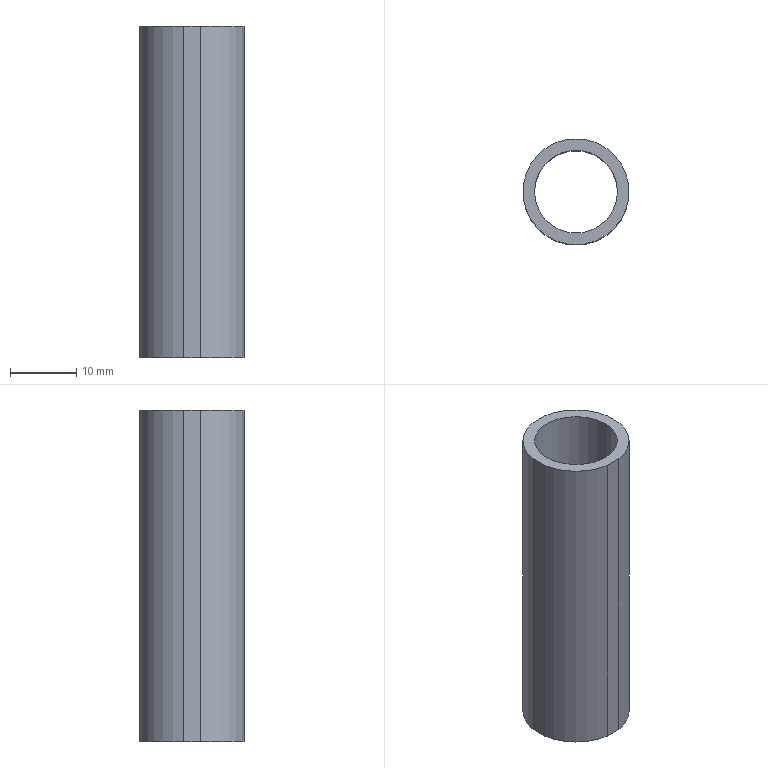Part | SolidWorks | features Extrusion 1, ICE 1 | 1 solid | 12 faces | box 15.8 x 15.8 x 50 mm | volume 3884 mm3 | cylinder 6 | plane 6 | commonest cylinder face diameters 16 x4 12.5 x2
STEP:
#1=CARTESIAN_POINT('',(-6.25,0.,50.));
#2=VERTEX_POINT('',#1);
#3=CARTESIAN_POINT('',(6.25,0.,50.));
#4=VERTEX_POINT('',#3);
#5=CARTESIAN_POINT('',(0.,0.,50.));
#6=DIRECTION('',(0.,0.,1.));
#7=DIRECTION('',(1.,0.,0.));
#8=AXIS2_PLACEMENT_3D('',#5,#6,#7);
#9=CIRCLE('',#8,6.25);
#10=EDGE_CURVE('',#2,#4,#9,.T.);
#11=ORIENTED_EDGE('',*,*,#10,.T.);
#12=CARTESIAN_POINT('',(6.25,0.,0.));
#13=VERTEX_POINT('',#12);
#14=CARTESIAN_POINT('',(6.25,0.,50.));
#15=DIRECTION('',(0.,0.,-1.));
#16=VECTOR('',#15,1000.);
#17=LINE('',#14,#16);
#18=EDGE_CURVE('',#4,#13,#17,.T.);
#19=ORIENTED_EDGE('',*,*,#18,.T.);
#20=CARTESIAN_POINT('',(-6.25,0.,0.));
#21=VERTEX_POINT('',#20);
#22=CARTESIAN_POINT('',(0.,0.,0.));
#23=DIRECTION('',(0.,0.,1.));
#24=DIRECTION('',(1.,0.,0.));
#25=AXIS2_PLACEMENT_3D('',#22,#23,#24);
#26=CIRCLE('',#25,6.25);
#27=EDGE_CURVE('',#21,#13,#26,.T.);
#28=ORIENTED_EDGE('',*,*,#27,.F.);
#29=CARTESIAN_POINT('',(-6.25,0.,50.));
#30=DIRECTION('',(0.,0.,-1.));
#31=VECTOR('',#30,1000.);
#32=LINE('',#29,#31);
#33=EDGE_CURVE('',#2,#21,#32,.T.);
#34=ORIENTED_EDGE('',*,*,#33,.F.);
#35=EDGE_LOOP('',(#11,#19,#28,#34));
#36=FACE_OUTER_BOUND('',#35,.T.);
#37=CARTESIAN_POINT('',(0.,0.,50.));
#38=DIRECTION('',(0.,0.,-1.));
#39=DIRECTION('',(-1.,0.,0.));
#40=AXIS2_PLACEMENT_3D('',#37,#38,#39);
#41=CYLINDRICAL_SURFACE('',#40,6.25);
#42=ADVANCED_FACE('',(#36),#41,.F.);
#43=ORIENTED_EDGE('',*,*,#10,.F.);
#44=CARTESIAN_POINT('',(0.,0.,50.));
#45=DIRECTION('',(0.,0.,1.));
#46=DIRECTION('',(1.,0.,0.));
#47=AXIS2_PLACEMENT_3D('',#44,#45,#46);
#48=CIRCLE('',#47,6.25);
#49=EDGE_CURVE('',#4,#2,#48,.T.);
#50=ORIENTED_EDGE('',*,*,#49,.F.);
#51=EDGE_LOOP('',(#43,#50));
#52=FACE_BOUND('',#51,.T.);
#53=CARTESIAN_POINT('',(-1.261,7.9,50.));
#54=VERTEX_POINT('',#53);
#55=CARTESIAN_POINT('',(-7.9,1.261,50.));
#56=VERTEX_POINT('',#55);
#57=CARTESIAN_POINT('',(0.,0.,50.));
#58=DIRECTION('',(0.,0.,1.));
#59=DIRECTION('',(1.,0.,0.));
#60=AXIS2_PLACEMENT_3D('',#57,#58,#59);
#61=CIRCLE('',#60,8.);
#62=EDGE_CURVE('',#54,#56,#61,.T.);
#63=ORIENTED_EDGE('',*,*,#62,.T.);
#64=CARTESIAN_POINT('',(-7.9,-1.261,50.));
#65=VERTEX_POINT('',#64);
#66=CARTESIAN_POINT('',(-7.9,7.9,50.));
#67=DIRECTION('',(0.,-1.,0.));
#68=VECTOR('',#67,1000.);
#69=LINE('',#66,#68);
#70=EDGE_CURVE('',#56,#65,#69,.T.);
#71=ORIENTED_EDGE('',*,*,#70,.T.);
#72=CARTESIAN_POINT('',(-1.261,-7.9,50.));
#73=VERTEX_POINT('',#72);
#74=CARTESIAN_POINT('',(0.,0.,50.));
#75=DIRECTION('',(0.,0.,1.));
#76=DIRECTION('',(1.,0.,0.));
#77=AXIS2_PLACEMENT_3D('',#74,#75,#76);
#78=CIRCLE('',#77,8.);
#79=EDGE_CURVE('',#65,#73,#78,.T.);
#80=ORIENTED_EDGE('',*,*,#79,.T.);
#81=CARTESIAN_POINT('',(1.261,-7.9,50.));
#82=VERTEX_POINT('',#81);
#83=CARTESIAN_POINT('',(7.9,-7.9,50.));
#84=DIRECTION('',(1.,0.,0.));
#85=VECTOR('',#84,1000.);
#86=LINE('',#83,#85);
#87=EDGE_CURVE('',#73,#82,#86,.T.);
#88=ORIENTED_EDGE('',*,*,#87,.T.);
#89=CARTESIAN_POINT('',(7.9,-1.261,50.));
#90=VERTEX_POINT('',#89);
#91=CARTESIAN_POINT('',(0.,0.,50.));
#92=DIRECTION('',(0.,0.,1.));
#93=DIRECTION('',(1.,0.,0.));
#94=AXIS2_PLACEMENT_3D('',#91,#92,#93);
#95=CIRCLE('',#94,8.);
#96=EDGE_CURVE('',#82,#90,#95,.T.);
#97=ORIENTED_EDGE('',*,*,#96,.T.);
#98=CARTESIAN_POINT('',(7.9,1.261,50.));
#99=VERTEX_POINT('',#98);
#100=CARTESIAN_POINT('',(7.9,7.9,50.));
#101=DIRECTION('',(0.,1.,0.));
#102=VECTOR('',#101,1000.);
#103=LINE('',#100,#102);
#104=EDGE_CURVE('',#90,#99,#103,.T.);
#105=ORIENTED_EDGE('',*,*,#104,.T.);
#106=CARTESIAN_POINT('',(1.261,7.9,50.));
#107=VERTEX_POINT('',#106);
#108=CARTESIAN_POINT('',(0.,0.,50.));
#109=DIRECTION('',(0.,0.,1.));
#110=DIRECTION('',(1.,0.,0.));
#111=AXIS2_PLACEMENT_3D('',#108,#109,#110);
#112=CIRCLE('',#111,8.);
#113=EDGE_CURVE('',#99,#107,#112,.T.);
#114=ORIENTED_EDGE('',*,*,#113,.T.);
#115=CARTESIAN_POINT('',(7.9,7.9,50.));
#116=DIRECTION('',(-1.,0.,0.));
#117=VECTOR('',#116,1000.);
#118=LINE('',#115,#117);
#119=EDGE_CURVE('',#107,#54,#118,.T.);
#120=ORIENTED_EDGE('',*,*,#119,.T.);
#121=EDGE_LOOP('',(#63,#71,#80,#88,#97,#105,#114,#120));
#122=FACE_OUTER_BOUND('',#121,.T.);
#123=CARTESIAN_POINT('',(0.,0.,50.));
#124=DIRECTION('',(0.,0.,1.));
#125=DIRECTION('',(1.,0.,0.));
#126=AXIS2_PLACEMENT_3D('',#123,#124,#125);
#127=PLANE('',#126);
#128=ADVANCED_FACE('',(#52,#122),#127,.T.);
#129=ORIENTED_EDGE('',*,*,#27,.T.);
#130=CARTESIAN_POINT('',(0.,0.,0.));
#131=DIRECTION('',(0.,0.,1.));
#132=DIRECTION('',(1.,0.,0.));
#133=AXIS2_PLACEMENT_3D('',#130,#131,#132);
#134=CIRCLE('',#133,6.25);
#135=EDGE_CURVE('',#13,#21,#134,.T.);
#136=ORIENTED_EDGE('',*,*,#135,.T.);
#137=EDGE_LOOP('',(#129,#136));
#138=FACE_BOUND('',#137,.T.);
#139=CARTESIAN_POINT('',(-7.9,1.261,0.));
#140=VERTEX_POINT('',#139);
#141=CARTESIAN_POINT('',(-7.9,-1.261,0.));
#142=VERTEX_POINT('',#141);
#143=CARTESIAN_POINT('',(-7.9,7.9,0.));
#144=DIRECTION('',(0.,-1.,0.));
#145=VECTOR('',#144,1000.);
#146=LINE('',#143,#145);
#147=EDGE_CURVE('',#140,#142,#146,.T.);
#148=ORIENTED_EDGE('',*,*,#147,.F.);
#149=CARTESIAN_POINT('',(-1.261,7.9,0.));
#150=VERTEX_POINT('',#149);
#151=CARTESIAN_POINT('',(0.,0.,0.));
#152=DIRECTION('',(0.,0.,1.));
#153=DIRECTION('',(1.,0.,0.));
#154=AXIS2_PLACEMENT_3D('',#151,#152,#153);
#155=CIRCLE('',#154,8.);
#156=EDGE_CURVE('',#150,#140,#155,.T.);
#157=ORIENTED_EDGE('',*,*,#156,.F.);
#158=CARTESIAN_POINT('',(1.261,7.9,0.));
#159=VERTEX_POINT('',#158);
#160=CARTESIAN_POINT('',(7.9,7.9,0.));
#161=DIRECTION('',(-1.,0.,0.));
#162=VECTOR('',#161,1000.);
#163=LINE('',#160,#162);
#164=EDGE_CURVE('',#159,#150,#163,.T.);
#165=ORIENTED_EDGE('',*,*,#164,.F.);
#166=CARTESIAN_POINT('',(7.9,1.261,0.));
#167=VERTEX_POINT('',#166);
#168=CARTESIAN_POINT('',(0.,0.,0.));
#169=DIRECTION('',(0.,0.,1.));
#170=DIRECTION('',(1.,0.,0.));
#171=AXIS2_PLACEMENT_3D('',#168,#169,#170);
#172=CIRCLE('',#171,8.);
#173=EDGE_CURVE('',#167,#159,#172,.T.);
#174=ORIENTED_EDGE('',*,*,#173,.F.);
#175=CARTESIAN_POINT('',(7.9,-1.261,0.));
#176=VERTEX_POINT('',#175);
#177=CARTESIAN_POINT('',(7.9,7.9,0.));
#178=DIRECTION('',(0.,1.,0.));
#179=VECTOR('',#178,1000.);
#180=LINE('',#177,#179);
#181=EDGE_CURVE('',#176,#167,#180,.T.);
#182=ORIENTED_EDGE('',*,*,#181,.F.);
#183=CARTESIAN_POINT('',(1.261,-7.9,0.));
#184=VERTEX_POINT('',#183);
#185=CARTESIAN_POINT('',(0.,0.,0.));
#186=DIRECTION('',(0.,0.,1.));
#187=DIRECTION('',(1.,0.,0.));
#188=AXIS2_PLACEMENT_3D('',#185,#186,#187);
#189=CIRCLE('',#188,8.);
#190=EDGE_CURVE('',#184,#176,#189,.T.);
#191=ORIENTED_EDGE('',*,*,#190,.F.);
#192=CARTESIAN_POINT('',(-1.261,-7.9,0.));
#193=VERTEX_POINT('',#192);
#194=CARTESIAN_POINT('',(7.9,-7.9,0.));
#195=DIRECTION('',(1.,0.,0.));
#196=VECTOR('',#195,1000.);
#197=LINE('',#194,#196);
#198=EDGE_CURVE('',#193,#184,#197,.T.);
#199=ORIENTED_EDGE('',*,*,#198,.F.);
#200=CARTESIAN_POINT('',(0.,0.,0.));
#201=DIRECTION('',(0.,0.,1.));
#202=DIRECTION('',(1.,0.,0.));
#203=AXIS2_PLACEMENT_3D('',#200,#201,#202);
#204=CIRCLE('',#203,8.);
#205=EDGE_CURVE('',#142,#193,#204,.T.);
#206=ORIENTED_EDGE('',*,*,#205,.F.);
#207=EDGE_LOOP('',(#148,#157,#165,#174,#182,#191,#199,#206));
#208=FACE_OUTER_BOUND('',#207,.T.);
#209=CARTESIAN_POINT('',(0.,0.,0.));
#210=DIRECTION('',(0.,0.,1.));
#211=DIRECTION('',(1.,0.,0.));
#212=AXIS2_PLACEMENT_3D('',#209,#210,#211);
#213=PLANE('',#212);
#214=ADVANCED_FACE('',(#138,#208),#213,.F.);
#215=CARTESIAN_POINT('',(-7.9,1.261,50.));
#216=DIRECTION('',(0.,0.,-1.));
#217=VECTOR('',#216,1000.);
#218=LINE('',#215,#217);
#219=EDGE_CURVE('',#56,#140,#218,.T.);
#220=ORIENTED_EDGE('',*,*,#219,.F.);
#221=ORIENTED_EDGE('',*,*,#62,.F.);
#222=CARTESIAN_POINT('',(-1.261,7.9,50.));
#223=DIRECTION('',(0.,0.,1.));
#224=VECTOR('',#223,1000.);
#225=LINE('',#222,#224);
#226=EDGE_CURVE('',#150,#54,#225,.T.);
#227=ORIENTED_EDGE('',*,*,#226,.F.);
#228=ORIENTED_EDGE('',*,*,#156,.T.);
#229=EDGE_LOOP('',(#220,#221,#227,#228));
#230=FACE_OUTER_BOUND('',#229,.T.);
#231=CARTESIAN_POINT('',(0.,0.,50.));
#232=DIRECTION('',(0.,0.,-1.));
#233=DIRECTION('',(-1.,0.,0.));
#234=AXIS2_PLACEMENT_3D('',#231,#232,#233);
#235=CYLINDRICAL_SURFACE('',#234,8.);
#236=ADVANCED_FACE('',(#230),#235,.T.);
#237=CARTESIAN_POINT('',(-7.9,-1.261,50.));
#238=DIRECTION('',(0.,0.,1.));
#239=VECTOR('',#238,1000.);
#240=LINE('',#237,#239);
#241=EDGE_CURVE('',#142,#65,#240,.T.);
#242=ORIENTED_EDGE('',*,*,#241,.F.);
#243=ORIENTED_EDGE('',*,*,#205,.T.);
#244=CARTESIAN_POINT('',(-1.261,-7.9,50.));
#245=DIRECTION('',(0.,0.,-1.));
#246=VECTOR('',#245,1000.);
#247=LINE('',#244,#246);
#248=EDGE_CURVE('',#73,#193,#247,.T.);
#249=ORIENTED_EDGE('',*,*,#248,.F.);
#250=ORIENTED_EDGE('',*,*,#79,.F.);
#251=EDGE_LOOP('',(#242,#243,#249,#250));
#252=FACE_OUTER_BOUND('',#251,.T.);
#253=CARTESIAN_POINT('',(0.,0.,50.));
#254=DIRECTION('',(0.,0.,-1.));
#255=DIRECTION('',(-1.,0.,0.));
#256=AXIS2_PLACEMENT_3D('',#253,#254,#255);
#257=CYLINDRICAL_SURFACE('',#256,8.);
#258=ADVANCED_FACE('',(#252),#257,.T.);
#259=CARTESIAN_POINT('',(1.261,7.9,50.));
#260=DIRECTION('',(0.,0.,-1.));
#261=VECTOR('',#260,1000.);
#262=LINE('',#259,#261);
#263=EDGE_CURVE('',#107,#159,#262,.T.);
#264=ORIENTED_EDGE('',*,*,#263,.F.);
#265=ORIENTED_EDGE('',*,*,#113,.F.);
#266=CARTESIAN_POINT('',(7.9,1.261,50.));
#267=DIRECTION('',(0.,0.,1.));
#268=VECTOR('',#267,1000.);
#269=LINE('',#266,#268);
#270=EDGE_CURVE('',#167,#99,#269,.T.);
#271=ORIENTED_EDGE('',*,*,#270,.F.);
#272=ORIENTED_EDGE('',*,*,#173,.T.);
#273=EDGE_LOOP('',(#264,#265,#271,#272));
#274=FACE_OUTER_BOUND('',#273,.T.);
#275=CARTESIAN_POINT('',(0.,0.,50.));
#276=DIRECTION('',(0.,0.,-1.));
#277=DIRECTION('',(-1.,0.,0.));
#278=AXIS2_PLACEMENT_3D('',#275,#276,#277);
#279=CYLINDRICAL_SURFACE('',#278,8.);
#280=ADVANCED_FACE('',(#274),#279,.T.);
#281=CARTESIAN_POINT('',(7.9,-1.261,50.));
#282=DIRECTION('',(0.,0.,-1.));
#283=VECTOR('',#282,1000.);
#284=LINE('',#281,#283);
#285=EDGE_CURVE('',#90,#176,#284,.T.);
#286=ORIENTED_EDGE('',*,*,#285,.F.);
#287=ORIENTED_EDGE('',*,*,#96,.F.);
#288=CARTESIAN_POINT('',(1.261,-7.9,50.));
#289=DIRECTION('',(0.,0.,1.));
#290=VECTOR('',#289,1000.);
#291=LINE('',#288,#290);
#292=EDGE_CURVE('',#184,#82,#291,.T.);
#293=ORIENTED_EDGE('',*,*,#292,.F.);
#294=ORIENTED_EDGE('',*,*,#190,.T.);
#295=EDGE_LOOP('',(#286,#287,#293,#294));
#296=FACE_OUTER_BOUND('',#295,.T.);
#297=CARTESIAN_POINT('',(0.,0.,50.));
#298=DIRECTION('',(0.,0.,-1.));
#299=DIRECTION('',(-1.,0.,0.));
#300=AXIS2_PLACEMENT_3D('',#297,#298,#299);
#301=CYLINDRICAL_SURFACE('',#300,8.);
#302=ADVANCED_FACE('',(#296),#301,.T.);
#303=ORIENTED_EDGE('',*,*,#18,.F.);
#304=ORIENTED_EDGE('',*,*,#49,.T.);
#305=ORIENTED_EDGE('',*,*,#33,.T.);
#306=ORIENTED_EDGE('',*,*,#135,.F.);
#307=EDGE_LOOP('',(#303,#304,#305,#306));
#308=FACE_OUTER_BOUND('',#307,.T.);
#309=CARTESIAN_POINT('',(0.,0.,50.));
#310=DIRECTION('',(0.,0.,-1.));
#311=DIRECTION('',(-1.,0.,0.));
#312=AXIS2_PLACEMENT_3D('',#309,#310,#311);
#313=CYLINDRICAL_SURFACE('',#312,6.25);
#314=ADVANCED_FACE('',(#308),#313,.F.);
#315=ORIENTED_EDGE('',*,*,#248,.T.);
#316=ORIENTED_EDGE('',*,*,#198,.T.);
#317=ORIENTED_EDGE('',*,*,#292,.T.);
#318=ORIENTED_EDGE('',*,*,#87,.F.);
#319=EDGE_LOOP('',(#315,#316,#317,#318));
#320=FACE_OUTER_BOUND('',#319,.T.);
#321=CARTESIAN_POINT('',(7.9,-7.9,0.));
#322=DIRECTION('',(0.,-1.,0.));
#323=DIRECTION('',(1.,0.,0.));
#324=AXIS2_PLACEMENT_3D('',#321,#322,#323);
#325=PLANE('',#324);
#326=ADVANCED_FACE('',(#320),#325,.T.);
#327=ORIENTED_EDGE('',*,*,#285,.T.);
#328=ORIENTED_EDGE('',*,*,#181,.T.);
#329=ORIENTED_EDGE('',*,*,#270,.T.);
#330=ORIENTED_EDGE('',*,*,#104,.F.);
#331=EDGE_LOOP('',(#327,#328,#329,#330));
#332=FACE_OUTER_BOUND('',#331,.T.);
#333=CARTESIAN_POINT('',(7.9,7.9,0.));
#334=DIRECTION('',(1.,0.,0.));
#335=DIRECTION('',(0.,1.,0.));
#336=AXIS2_PLACEMENT_3D('',#333,#334,#335);
#337=PLANE('',#336);
#338=ADVANCED_FACE('',(#332),#337,.T.);
#339=ORIENTED_EDGE('',*,*,#263,.T.);
#340=ORIENTED_EDGE('',*,*,#164,.T.);
#341=ORIENTED_EDGE('',*,*,#226,.T.);
#342=ORIENTED_EDGE('',*,*,#119,.F.);
#343=EDGE_LOOP('',(#339,#340,#341,#342));
#344=FACE_OUTER_BOUND('',#343,.T.);
#345=CARTESIAN_POINT('',(7.9,7.9,0.));
#346=DIRECTION('',(0.,1.,0.));
#347=DIRECTION('',(-1.,0.,0.));
#348=AXIS2_PLACEMENT_3D('',#345,#346,#347);
#349=PLANE('',#348);
#350=ADVANCED_FACE('',(#344),#349,.T.);
#351=ORIENTED_EDGE('',*,*,#219,.T.);
#352=ORIENTED_EDGE('',*,*,#147,.T.);
#353=ORIENTED_EDGE('',*,*,#241,.T.);
#354=ORIENTED_EDGE('',*,*,#70,.F.);
#355=EDGE_LOOP('',(#351,#352,#353,#354));
#356=FACE_OUTER_BOUND('',#355,.T.);
#357=CARTESIAN_POINT('',(-7.9,7.9,0.));
#358=DIRECTION('',(-1.,0.,0.));
#359=DIRECTION('',(0.,-1.,0.));
#360=AXIS2_PLACEMENT_3D('',#357,#358,#359);
#361=PLANE('',#360);
#362=ADVANCED_FACE('',(#356),#361,.T.);
#363=CLOSED_SHELL('',(#42,#128,#214,#236,#258,#280,#302,#314,#326,#338,#350,#362));
#364=MANIFOLD_SOLID_BREP('',#363);
#365=CARTESIAN_POINT('',(0.,0.,0.));
#366=DIRECTION('',(0.,0.,1.));
#367=DIRECTION('',(1.,0.,0.));
#368=AXIS2_PLACEMENT_3D('',#365,#366,#367);
#369=(LENGTH_UNIT()NAMED_UNIT(*)SI_UNIT(.MILLI.,.METRE.));
#370=UNCERTAINTY_MEASURE_WITH_UNIT(LENGTH_MEASURE(0.00001),#369,'','');
#371=(NAMED_UNIT(*)PLANE_ANGLE_UNIT()SI_UNIT($,.RADIAN.));
#372=(NAMED_UNIT(*)SI_UNIT($,.STERADIAN.)SOLID_ANGLE_UNIT());
#373=(GEOMETRIC_REPRESENTATION_CONTEXT(3)GLOBAL_UNCERTAINTY_ASSIGNED_CONTEXT((#370))GLOBAL_UNIT_ASSIGNED_CONTEXT((#369,#371,#372))REPRESENTATION_CONTEXT('',''));
#374=ADVANCED_BREP_SHAPE_REPRESENTATION('',(#364,#368),#373);